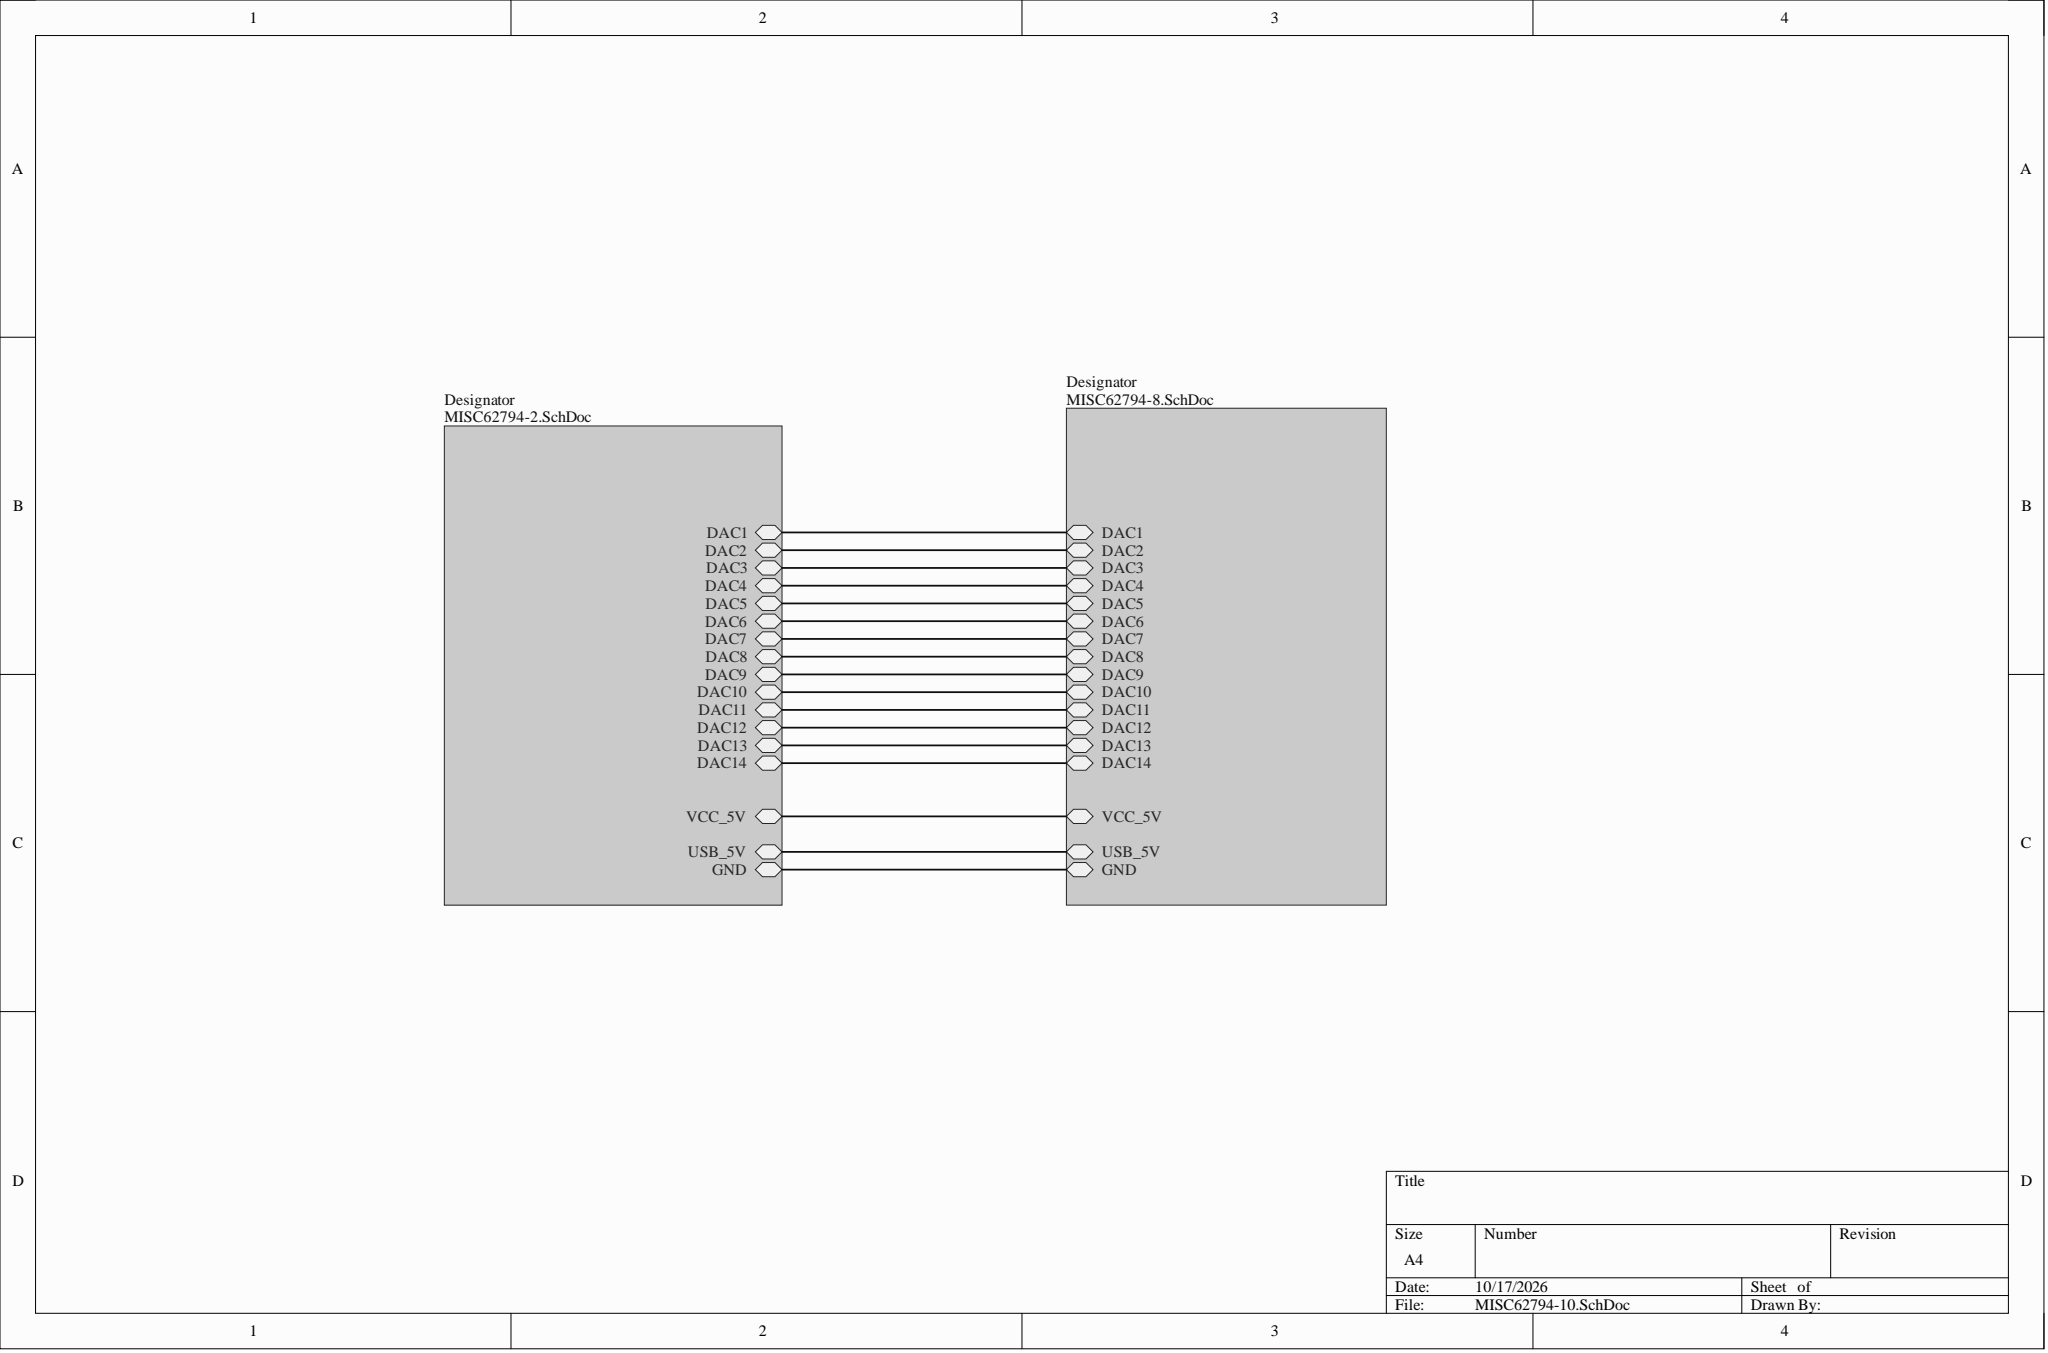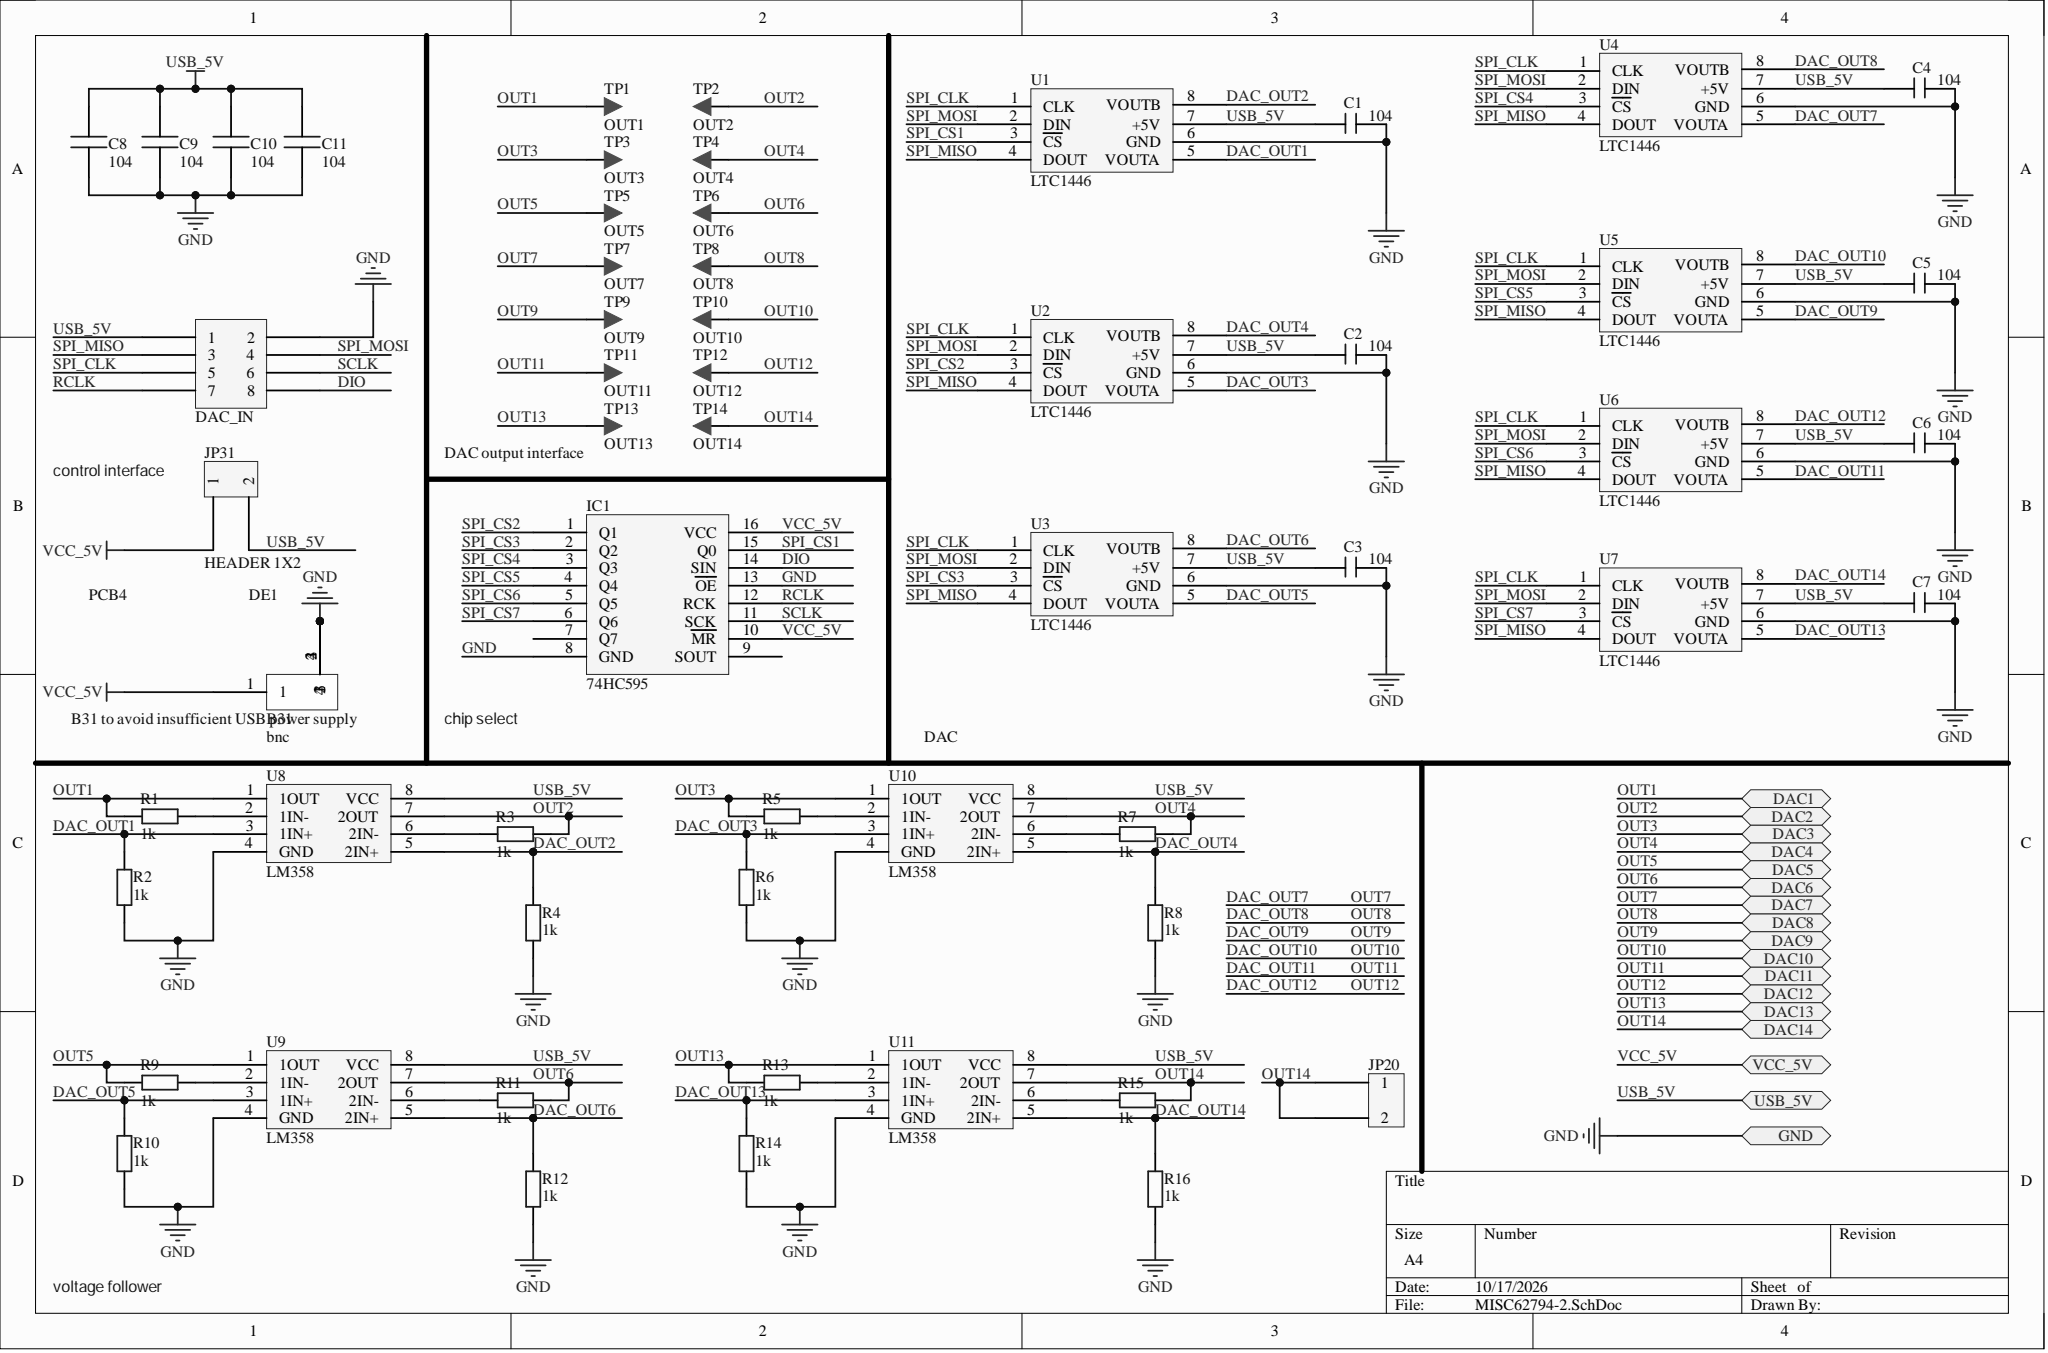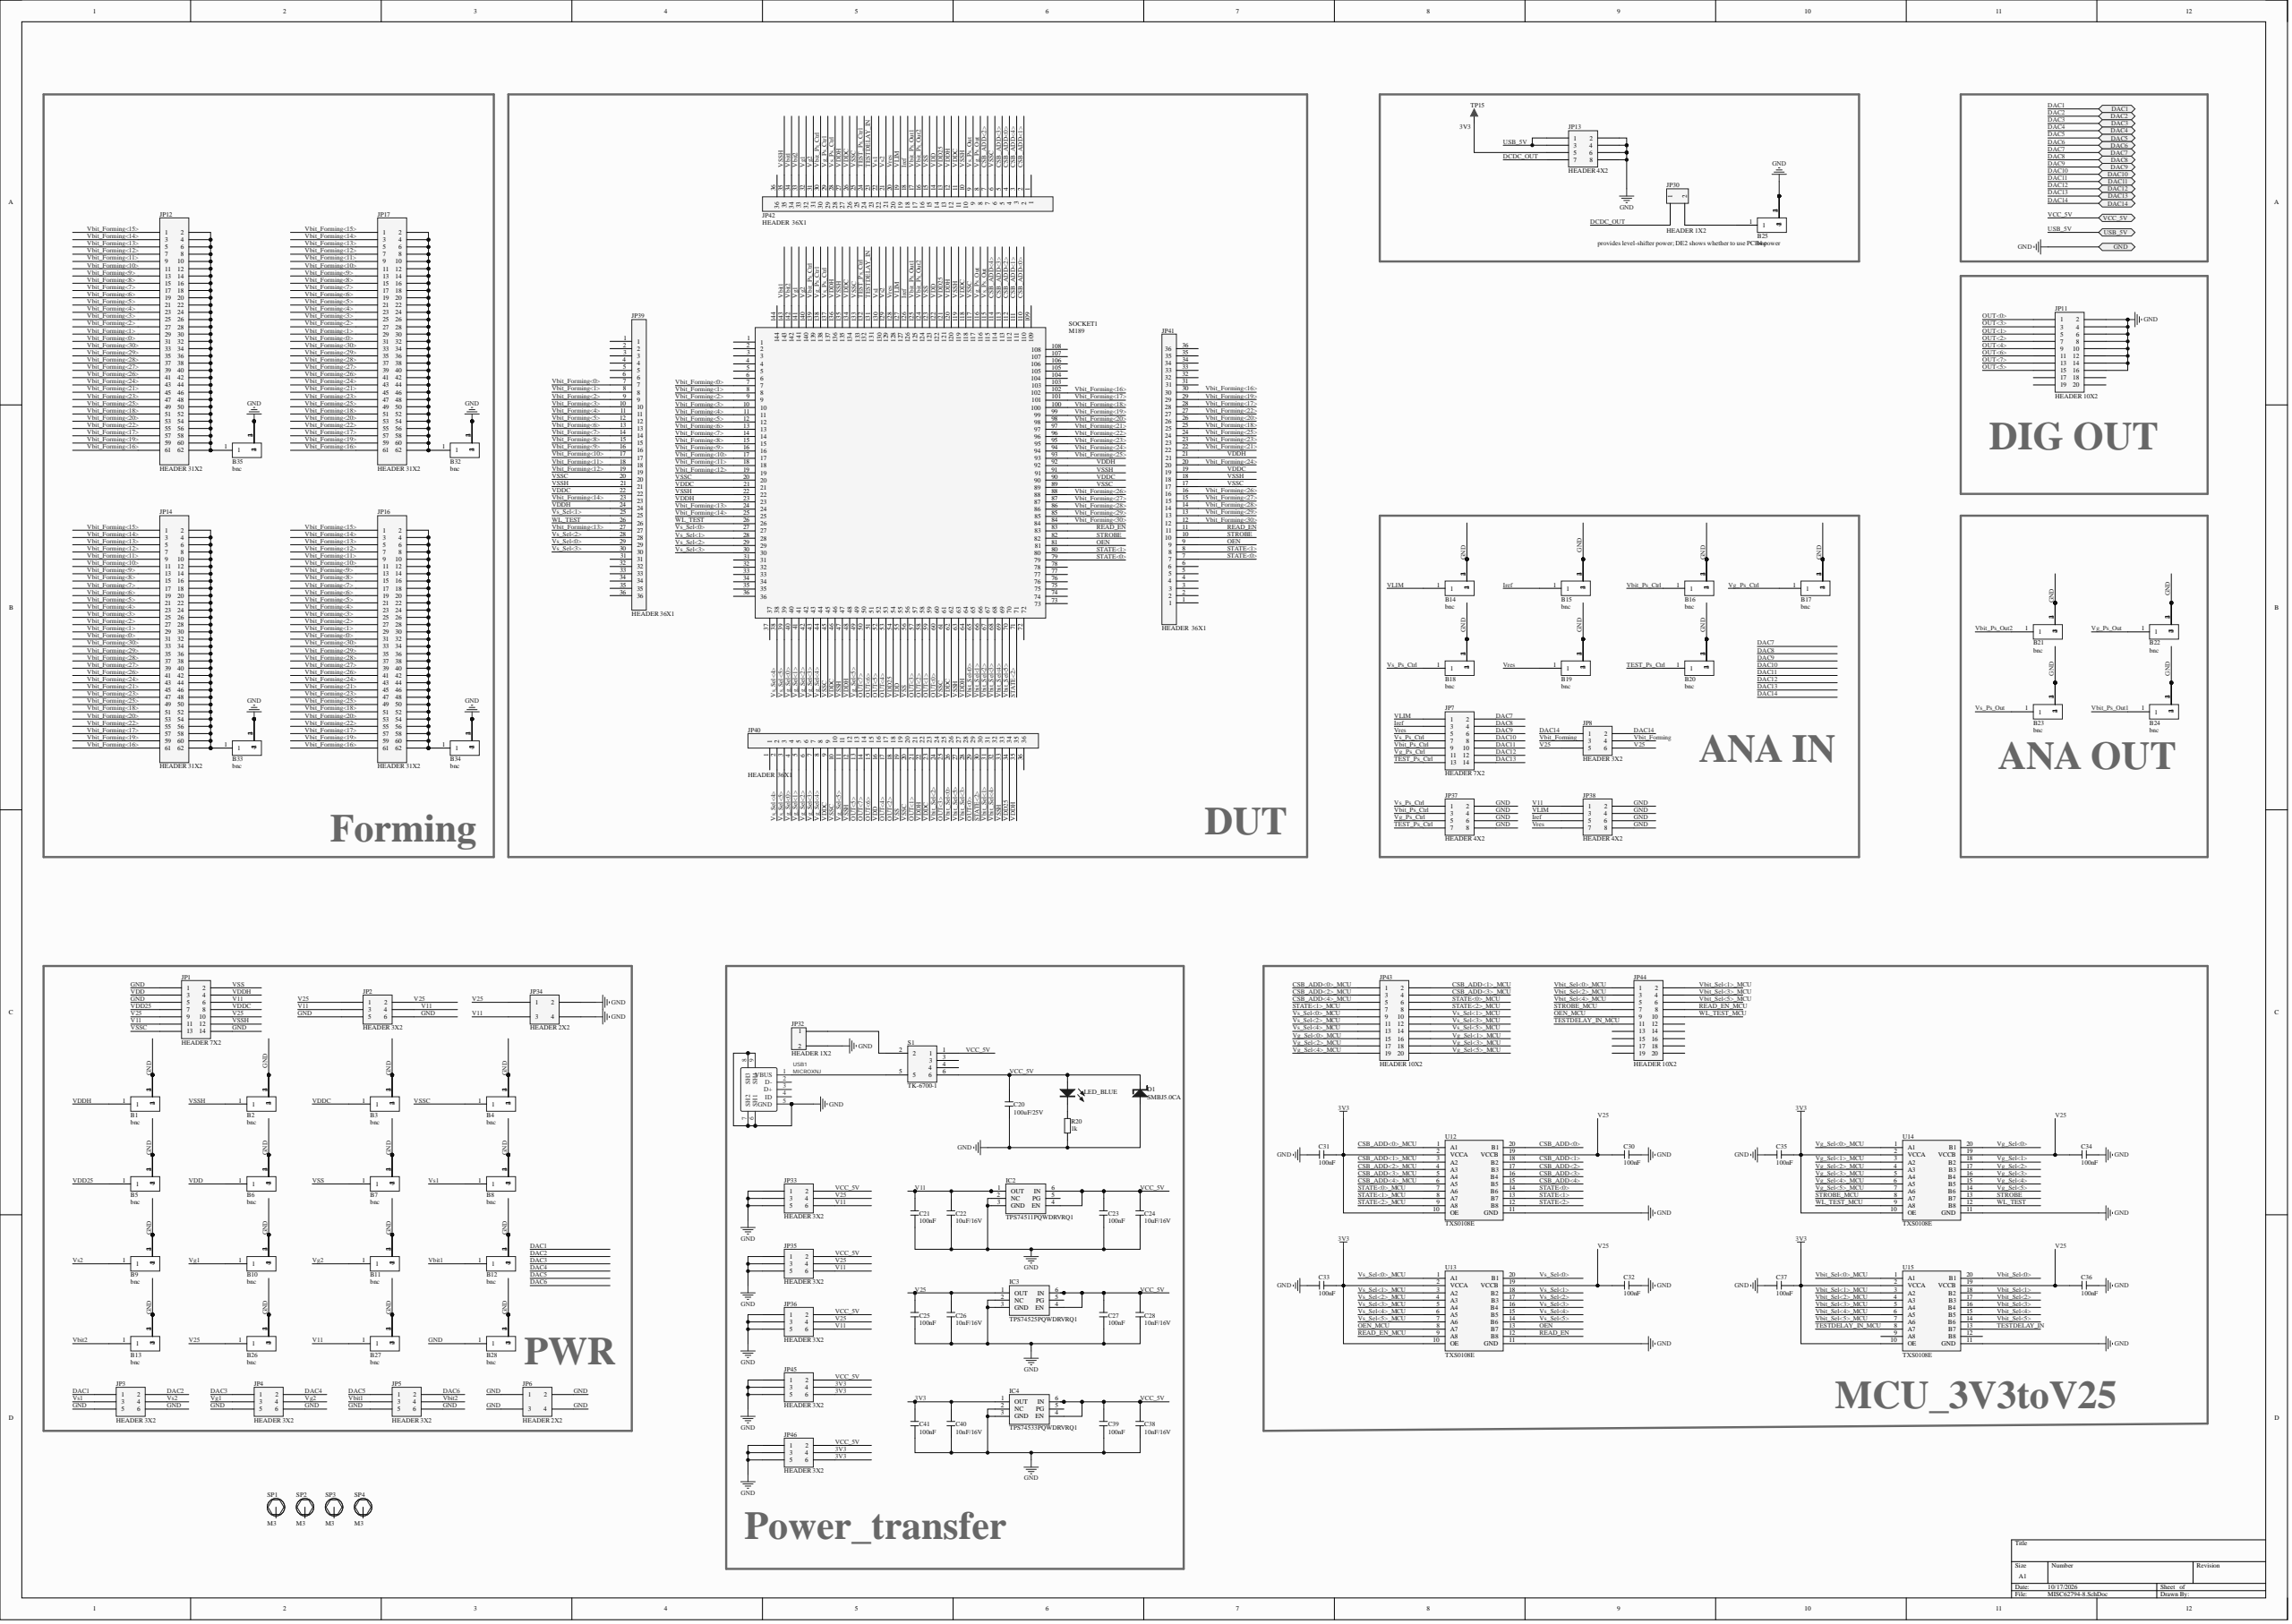Circuit board | Altium Designer | 158 parts | 185 nets
Bill of materials:
Comment,Description,Designator,Footprint,LibRef,Quantity
"bnc","bnc","B1, B2, B3, B4, B5, B6, B7, B8, B9, B10, B11, B12, B13, B14, B15, B16, B17, B18, B19, B20, B21, B22, B23, B24, B25, B26, B27, B28, B31, B32, B33, B34, B35","BNC-TH_DOSIN-801-0072","bnc","33"
"104","capacitor model","C1, C2, C3, C4, C5, C6, C7, C8, C9, C10, C11","0603C","CAP","11"
"100uF/25V","capacitor model","C20","EC-D6.3x7.7","CAP","1"
"100nF","capacitor model","C21, C23, C25, C27, C30, C31, C32, C33, C34, C35, C36, C37, C39, C41","0603C","CAP","14"
"10uF/16V","capacitor model","C22, C24","0603C","CAP","2"
"10nF/16V","capacitor model","C26, C28, C38, C40","0603C","CAP","4"
"SMBJ5.0CA","diode","D1","SMB","SMBJ5.0CA","1"
"DAC_IN","DAC_IN","DAC_IN","HDR2.54-LI-2x4P","DAC_IN","1"
"74HC595","IC","IC1","SOIC-16_L9.9-W3.9-P1.27-LS6.0-BL","74HC595","1"
"TPS74511PQWDRVRQ1","LDO","IC2","WSON-6_L2.0-W2.0-P0.65-BL-EP","TPS74511PQWDRVRQ1","1"
"TPS74525PQWDRVRQ1","LDO","IC3","WSON-6_L2.0-W2.0-P0.65-BL-EP","TPS74525PQWDRVRQ1","1"
"TPS74533PQWDRVRQ1","LDO","IC4","WSON-6_L2.0-W2.0-P0.65-BL-EP","TPS74533PQWDRVRQ1","1"
"HEADER 7X2","pin header","JP1, JP7","HDR2.54-LI-2x7P","HEADER 7X2","2"
"HEADER 3X2","pin header","JP2, JP3, JP4, JP5, JP8, JP33, JP35, JP36, JP45, JP46","HDR2.54-LI-2x3P","HEADER 3X2","10"
"HEADER 2X2","pin header","JP6","HDR2.54-LI-2x3P","HEADER 2X2","1"
"HEADER 10X2","pin header","JP11, JP43, JP44","HDR2.54-LI-2x10P","HEADER 10X2","3"
"HEADER 31X2","pin header","JP12, JP14, JP16, JP17","HDR2.54-LI-2x31P","HEADER 31X2","4"
"HEADER 4X2","pin header","JP13, JP37, JP38","HDR2.54-LI-2x4P","HEADER 4X2","3"
"HEADER 1X2","pin header","JP20, JP30, JP31, JP32","HDR2.54-LI-2P","HEADER 1X2","4"
"HEADER 2X2","pin header","JP34","HDR2.54-LI-2x2P","HEADER 2X2","1"
"HEADER 36X1","pin header","JP39","HDR2.54-LI-1x36P","HEADER 36X1","1"
"HEADER  36X1","pin header","JP40, JP41, JP42","HDR2.54-LI-1x36P","HEADER 36X1","3"
"LED","light-emitting diode","LED_BLUE","LED0805-R-RD","LED","1"
"1k","resistor model","R1, R2, R3, R4, R5, R6, R7, R8, R9, R10, R11, R12, R13, R14, R15, R16, R20","0603R","RES","17"
"TK-6700-1","six-pin self-locking switch","S1","SW-TH_6P-L8.0-W8.0-P2.50","switch6","1"
"M189","array","SOCKET1","YAMAICHI_IC51-1444-1354-7","M189_4K","1"
"M3","M3 interface","SP1, SP2, SP3, SP4","M3","M3","4"
"OUT1","TP","TP1","TP1.0","TP","1"
"OUT2","TP","TP2","TP1.0","TP","1"
"OUT3","TP","TP3","TP1.0","TP","1"
"OUT4","TP","TP4","TP1.0","TP","1"
"OUT5","TP","TP5","TP1.0","TP","1"
"OUT6","TP","TP6","TP1.0","TP","1"
"OUT7","TP","TP7","TP1.0","TP","1"
"OUT8","TP","TP8","TP1.0","TP","1"
"OUT9","TP","TP9","TP1.0","TP","1"
"OUT10","TP","TP10","TP1.0","TP","1"
"OUT11","TP","TP11","TP1.0","TP","1"
"OUT12","TP","TP12","TP1.0","TP","1"
"OUT13","TP","TP13","TP1.0","TP","1"
"OUT14","TP","TP14","TP1.0","TP","1"
"3V3","TP","TP15","TP1.0","TP","1"
"LTC1446","IC","U1, U2, U3, U4, U5, U6, U7","SO-8","LTC1446","7"
"LM358","IC","U8, U9, U10, U11","SO-8","LM358","4"
"TXS0108E","","U12, U13, U14, U15","TSSOP-20_L6.5-W4.4-P0.65-LS6.4-BL","TXS0108E","4"
"MICROXNJ","","USB1","MICRO-USB-SMD_MICROXNJ","MICROXNJ","1"
Netlist (Protel format):
[
B1
BNC-TH_DOSIN-801-0072
bnc



]
[
B2
BNC-TH_DOSIN-801-0072
bnc



]
[
B3
BNC-TH_DOSIN-801-0072
bnc



]
[
B4
BNC-TH_DOSIN-801-0072
bnc



]
[
B5
BNC-TH_DOSIN-801-0072
bnc



]
[
B6
BNC-TH_DOSIN-801-0072
bnc



]
[
B7
BNC-TH_DOSIN-801-0072
bnc



]
[
B8
BNC-TH_DOSIN-801-0072
bnc



]
[
B9
BNC-TH_DOSIN-801-0072
bnc



]
[
B10
BNC-TH_DOSIN-801-0072
bnc



]
[
B11
BNC-TH_DOSIN-801-0072
bnc



]
[
B12
BNC-TH_DOSIN-801-0072
bnc



]
[
B13
BNC-TH_DOSIN-801-0072
bnc



]
[
B14
BNC-TH_DOSIN-801-0072
bnc



]
[
B15
BNC-TH_DOSIN-801-0072
bnc



]
[
B16
BNC-TH_DOSIN-801-0072
bnc



]
[
B17
BNC-TH_DOSIN-801-0072
bnc



]
[
B18
BNC-TH_DOSIN-801-0072
bnc



]
[
B19
BNC-TH_DOSIN-801-0072
bnc



]
[
B20
BNC-TH_DOSIN-801-0072
bnc



]
[
B21
BNC-TH_DOSIN-801-0072
bnc



]
[
B22
BNC-TH_DOSIN-801-0072
bnc



]
[
B23
BNC-TH_DOSIN-801-0072
bnc



]
[
B24
BNC-TH_DOSIN-801-0072
bnc



]
[
B25
BNC-TH_DOSIN-801-0072
bnc



]
[
B26
BNC-TH_DOSIN-801-0072
bnc



]
[
B27
BNC-TH_DOSIN-801-0072
bnc



]
[
B28
BNC-TH_DOSIN-801-0072
bnc



]
[
B31
BNC-TH_DOSIN-801-0072
bnc



]
[
B32
BNC-TH_DOSIN-801-0072
bnc



]
[
B33
BNC-TH_DOSIN-801-0072
bnc



]
[
B34
BNC-TH_DOSIN-801-0072
bnc



]
[
B35
BNC-TH_DOSIN-801-0072
bnc



]
[
C1
0603C
104



]
[
C2
0603C
104



]
[
C3
0603C
104



]
[
C4
0603C
104



]
[
C5
0603C
104



]
[
C6
0603C
104



]
[
C7
0603C
104



]
[
C8
0603C
104



]
[
C9
0603C
104



]
[
C10
0603C
104



]
[
C11
0603C
104



]
[
C20
EC-D6.3x7.7
100uF/25V



]
[
C21
0603C
100nF



]
[
C22
0603C
10uF/16V



]
[
C23
0603C
100nF



]
[
C24
0603C
10uF/16V



]
[
C25
0603C
100nF



]
[
C26
0603C
10nF/16V



]
[
C27
0603C
100nF



]
[
C28
0603C
10nF/16V



]
[
C30
0603C
100nF



]
[
C31
0603C
100nF



]
[
C32
0603C
100nF



]
[
C33
0603C
100nF



]
[
C34
0603C
100nF



]
[
C35
0603C
100nF



]
[
C36
0603C
100nF



]
[
C37
0603C
100nF



]
[
C38
0603C
10nF/16V



]
[
C39
0603C
100nF



]
[
C40
0603C
10nF/16V



]
[
C41
0603C
100nF



]
[
D1
SMB
SMBJ5.0CA



]
[
DAC_IN
HDR2.54-LI-2x4P
DAC_IN



]
[
IC1
SOIC-16_L9.9-W3.9-P1.27-LS6.0-BL
74HC595



]
[
IC2
WSON-6_L2.0-W2.0-P0.65-BL-EP
TPS74511PQWDRVRQ1



]
[
IC3
WSON-6_L2.0-W2.0-P0.65-BL-EP
TPS74525PQWDRVRQ1



]
[
IC4
WSON-6_L2.0-W2.0-P0.65-BL-EP
TPS74533PQWDRVRQ1



]
[
JP1
HDR2.54-LI-2x7P
HEADER 7X2



]
[
JP2
HDR2.54-LI-2x3P
HEADER 3X2



]
[
JP3
HDR2.54-LI-2x3P
HEADER 3X2



]
[
JP4
HDR2.54-LI-2x3P
HEADER 3X2



]
[
JP5
HDR2.54-LI-2x3P
HEADER 3X2



]
[
JP6
HDR2.54-LI-2x3P
HEADER 2X2



]
[
JP7
HDR2.54-LI-2x7P
HEADER 7X2



]
[
JP8
HDR2.54-LI-2x3P
HEADER 3X2



]
[
JP11
HDR2.54-LI-2x10P
HEADER 10X2



]
[
JP12
HDR2.54-LI-2x31P
HEADER 31X2



]
[
JP13
HDR2.54-LI-2x4P
HEADER 4X2



]
[
JP14
HDR2.54-LI-2x31P
HEADER 31X2



]
[
JP16
HDR2.54-LI-2x31P
HEADER 31X2



]
[
JP17
HDR2.54-LI-2x31P
HEADER 31X2



]
[
JP20
HDR2.54-LI-2P
HEADER 1X2



]
[
JP30
HDR2.54-LI-2P
HEADER 1X2



]
[
JP31
HDR2.54-LI-2P
HEADER 1X2



]
[
JP32
HDR2.54-LI-2P
HEADER 1X2



]
[
JP33
HDR2.54-LI-2x3P
HEADER 3X2



]
[
JP34
HDR2.54-LI-2x2P
HEADER 2X2



]
[
JP35
HDR2.54-LI-2x3P
HEADER 3X2



]
[
JP36
HDR2.54-LI-2x3P
HEADER 3X2



]
[
JP37
HDR2.54-LI-2x4P
HEADER 4X2



]
[
JP38
HDR2.54-LI-2x4P
HEADER 4X2



]
[
JP39
HDR2.54-LI-1x36P
HEADER 36X1



]
[
JP40
HDR2.54-LI-1x36P
HEADER  36X1



]
[
JP41
HDR2.54-LI-1x36P
HEADER  36X1



]
[
JP42
HDR2.54-LI-1x36P
HEADER  36X1



]
[
JP43
HDR2.54-LI-2x10P
HEADER 10X2



]
[
JP44
HDR2.54-LI-2x10P
HEADER 10X2



]
[
JP45
HDR2.54-LI-2x3P
HEADER 3X2



]
[
JP46
HDR2.54-LI-2x3P
HEADER 3X2



]
[
LED_BLUE
LED0805-R-RD
LED



]
[
R1
0603R
1k



]
[
R2
0603R
1k



]
[
R3
0603R
1k



]
[
R4
0603R
1k



]
[
R5
0603R
1k



]
[
R6
0603R
1k



]
[
R7
0603R
1k



]
[
R8
0603R
1k



]
[
R9
0603R
1k



]
[
R10
0603R
1k



]
[
R11
0603R
1k



]
[
R12
0603R
1k



]
[
R13
0603R
1k



]
[
R14
0603R
1k



]
[
R15
0603R
1k



]
[
R16
0603R
1k



]
[
R20
0603R
1k



]
[
S1
SW-TH_6P-L8.0-W8.0-P2.50
TK-6700-1



]
[
SOCKET1
YAMAICHI_IC51-1444-1354-7
M189



]
[
SP1
M3
M3



]
[
SP2
M3
M3



]
[
SP3
M3
M3



]
[
SP4
M3
M3



]
[
TP1
TP1.0
OUT1



]
[
TP2
TP1.0
OUT2



]
[
TP3
TP1.0
OUT3



]
[
TP4
TP1.0
OUT4



]
[
TP5
TP1.0
OUT5



]
[
TP6
TP1.0
OUT6



]
[
TP7
TP1.0
OUT7



]
[
TP8
TP1.0
OUT8



]
[
TP9
TP1.0
OUT9



]
[
TP10
TP1.0
OUT10



]
[
TP11
TP1.0
OUT11



]
[
TP12
TP1.0
OUT12



]
[
TP13
TP1.0
OUT13



]
[
TP14
TP1.0
OUT14



]
[
TP15
TP1.0
3V3



]
[
U1
SO-8
LTC1446



]
[
U2
SO-8
LTC1446



]
[
U3
SO-8
LTC1446



]
[
U4
SO-8
LTC1446



]
[
U5
SO-8
LTC1446



]
[
U6
SO-8
LTC1446



]
[
U7
SO-8
LTC1446



]
[
U8
SO-8
LM358



]
[
U9
SO-8
LM358



]
[
U10
SO-8
LM358



]
[
U11
SO-8
LM358



]
[
U12
TSSOP-20_L6.5-W4.4-P0.65-LS6.4-BL
TXS0108E



]
[
U13
TSSOP-20_L6.5-W4.4-P0.65-LS6.4-BL
TXS0108E



]
[
U14
TSSOP-20_L6.5-W4.4-P0.65-LS6.4-BL
TXS0108E



]
[
U15
TSSOP-20_L6.5-W4.4-P0.65-LS6.4-BL
TXS0108E



]
[
USB1
MICRO-USB-SMD_MICROXNJ
MICROXNJ



]
(
WL_TEST_MCU
JP44-10
U14-9
)
(
WL_TEST
JP39-26
SOCKET1-26
U14-12
)
(
VSSH
B2-1
JP1-12
JP39-21
JP40-12
JP40-33
JP41-18
JP42-10
JP42-35
SOCKET1-22
SOCKET1-47
SOCKET1-63
SOCKET1-91
SOCKET1-119
SOCKET1-135
)
(
VSSC
B4-1
JP1-13
JP39-20
JP40-10
JP40-20
JP41-17
JP42-6
JP42-25
SOCKET1-20
SOCKET1-45
SOCKET1-61
SOCKET1-89
SOCKET1-117
SOCKET1-133
)
(
VSS
B7-1
JP1-2
JP40-19
JP42-15
SOCKET1-56
SOCKET1-123
)
(
Vs_Sel<5>_MCU
JP43-14
U13-7
)
(
Vs_Sel<5>
JP40-3
SOCKET1-39
U13-14
)
(
Vs_Sel<4>_MCU
JP43-13
U13-6
)
(
Vs_Sel<4>
JP40-2
SOCKET1-38
U13-15
)
(
Vs_Sel<3>_MCU
JP43-12
U13-5
)
(
Vs_Sel<3>
JP39-30
SOCKET1-30
U13-16
)
(
Vs_Sel<2>_MCU
JP43-11
U13-4
)
(
Vs_Sel<2>
JP39-28
SOCKET1-29
U13-17
)
(
Vs_Sel<1>_MCU
JP43-10
U13-3
)
(
Vs_Sel<1>
JP39-25
SOCKET1-28
U13-18
)
(
Vs_Sel<0>_MCU
JP43-9
U13-1
)
(
Vs_Sel<0>
JP39-29
SOCKET1-27
U13-20
)
(
Vs_Ps_Out
B23-1
JP42-9
SOCKET1-115
)
(
Vs_Ps_Ctrl
B18-1
JP7-7
JP37-1
JP42-28
SOCKET1-137
)
(
Vs2
B9-1
JP3-4
JP42-21
SOCKET1-129
)
(
Vs1
B8-1
JP3-3
JP42-22
SOCKET1-130
)
(
Vres
B19-1
JP7-5
JP38-7
JP42-20
SOCKET1-128
)
(
VLIM
B14-1
JP7-1
JP38-3
JP42-19
SOCKET1-127
)
(
Vg_Sel<5>_MCU
JP43-20
U14-7
)
(
Vg_Sel<5>
JP40-11
SOCKET1-49
U14-14
)
(
Vg_Sel<4>_MCU
JP43-19
U14-6
)
(
Vg_Sel<4>
JP40-8
SOCKET1-44
U14-15
)
(
Vg_Sel<3>_MCU
JP43-18
U14-5
)
(
Vg_Sel<3>
JP40-7
SOCKET1-43
U14-16
)
(
Vg_Sel<2>_MCU
JP43-17
U14-4
)
(
Vg_Sel<2>
JP40-6
SOCKET1-42
U14-17
)
(
Vg_Sel<1>_MCU
JP43-16
U14-3
)
(
Vg_Sel<1>
JP40-5
SOCKET1-41
U14-18
)
(
Vg_Sel<0>_MCU
JP43-15
U14-1
)
(
Vg_Sel<0>
JP40-4
SOCKET1-40
U14-20
)
(
Vg_Ps_Out
B22-1
JP42-8
SOCKET1-116
)
(
Vg_Ps_Ctrl
B17-1
JP7-11
JP37-5
JP42-29
SOCKET1-138
)
(
Vg2
B11-1
JP4-4
JP42-31
SOCKET1-140
)
(
Vg1
B10-1
JP4-3
JP42-32
SOCKET1-141
)
(
VDDH
B1-1
JP1-4
JP39-24
JP40-22
JP40-35
JP41-21
JP42-12
JP42-27
SOCKET1-23
SOCKET1-48
SOCKET1-64
SOCKET1-92
SOCKET1-120
SOCKET1-136
)
(
VDDC
B3-1
JP1-8
JP39-22
JP40-9
JP40-23
JP41-19
JP42-11
JP42-26
SOCKET1-21
SOCKET1-46
SOCKET1-62
SOCKET1-90
SOCKET1-118
SOCKET1-134
)
(
VDD25
B5-1
JP1-7
JP40-34
JP42-13
SOCKET1-54
SOCKET1-121
)
(
VDD
B6-1
JP1-3
JP40-16
JP42-14
SOCKET1-55
SOCKET1-122
)
(
VCC_5V
B31-1
C20-1
C23-1
C24-1
C27-1
C28-1
C38-1
C39-1
D1-1
IC1-10
IC1-16
IC2-4
IC2-6
IC3-4
IC3-6
IC4-4
IC4-6
JP31-1
JP33-2
JP35-2
JP36-2
JP45-2
JP46-2
LED_BLUE-1
S1-1
S1-6
)
(
Vbit_Sel<5>_MCU
JP44-6
U15-7
)
(
Vbit_Sel<5>
JP40-27
SOCKET1-70
U15-14
)
(
Vbit_Sel<4>_MCU
JP44-5
U15-6
)
(
Vbit_Sel<4>
JP40-32
SOCKET1-69
U15-15
)
(
Vbit_Sel<3>_MCU
JP44-4
U15-5
)
(
Vbit_Sel<3>
JP40-28
SOCKET1-68
U15-16
)
(
Vbit_Sel<2>_MCU
JP44-3
U15-4
)
(
Vbit_Sel<2>
JP40-24
SOCKET1-67
U15-17
)
(
Vbit_Sel<1>_MCU
JP44-2
U15-3
)
(
Vbit_Sel<1>
JP40-31
SOCKET1-66
U15-18
)
(
Vbit_Sel<0>_MCU
JP44-1
U15-1
)
(
Vbit_Sel<0>
JP40-26
SOCKET1-65
U15-20
)
(
Vbit_Ps_Out2
B21-1
JP42-16
SOCKET1-124
)
(
Vbit_Ps_Out1
B24-1
JP42-17
SOCKET1-125
)
(
Vbit_Ps_Ctrl
B16-1
JP7-9
JP37-3
JP42-30
SOCKET1-139
)
(
Vbit_Forming<30>
JP12-33
JP14-33
JP16-33
JP17-33
JP41-12
SOCKET1-84
)
(
Vbit_Forming<29>
JP12-35
JP14-35
JP16-35
JP17-35
JP41-13
SOCKET1-85
)
(
Vbit_Forming<28>
JP12-37
JP14-37
JP16-37
JP17-37
JP41-14
SOCKET1-86
)
(
Vbit_Forming<27>
JP12-39
JP14-39
JP16-39
JP17-39
JP41-15
SOCKET1-87
)
(
Vbit_Forming<26>
JP12-41
JP14-41
JP16-41
JP17-41
JP41-16
SOCKET1-88
)
(
Vbit_Forming<25>
JP12-49
JP14-49
JP16-49
JP17-49
JP41-24
SOCKET1-93
)
(
Vbit_Forming<24>
JP12-43
JP14-43
JP16-43
JP17-43
JP41-20
SOCKET1-94
)
(
Vbit_Forming<23>
JP12-47
JP14-47
JP16-47
JP17-47
JP41-23
SOCKET1-95
)
(
Vbit_Forming<22>
JP12-55
JP14-55
JP16-55
JP17-55
JP41-27
SOCKET1-96
)
(
Vbit_Forming<21>
JP12-45
JP14-45
JP16-45
JP17-45
JP41-22
SOCKET1-97
)
(
Vbit_Forming<20>
JP12-53
JP14-53
JP16-53
JP17-53
JP41-26
SOCKET1-98
)
(
Vbit_Forming<19>
JP12-59
JP14-59
JP16-59
JP17-59
JP41-29
SOCKET1-99
)
(
Vbit_Forming<18>
JP12-51
JP14-51
JP16-51
JP17-51
JP41-25
SOCKET1-100
)
(
Vbit_Forming<17>
JP12-57
JP14-57
JP16-57
JP17-57
JP41-28
SOCKET1-101
)
(
Vbit_Forming<16>
JP12-61
JP14-61
JP16-61
JP17-61
JP41-30
SOCKET1-102
)
(
Vbit_Forming<15>
JP12-1
JP14-1
JP16-1
JP17-1
)
(
Vbit_Forming<14>
JP12-3
JP14-3
JP16-3
JP17-3
JP39-23
SOCKET1-25
)
(
Vbit_Forming<13>
JP12-5
JP14-5
JP16-5
JP17-5
JP39-27
SOCKET1-24
)
(
Vbit_Forming<12>
JP12-7
JP14-7
JP16-7
JP17-7
JP39-19
SOCKET1-19
)
(
Vbit_Forming<11>
JP12-9
JP14-9
JP16-9
JP17-9
JP39-18
SOCKET1-18
)
(
Vbit_Forming<10>
JP12-11
JP14-11
JP16-11
JP17-11
JP39-17
SOCKET1-17
)
(
Vbit_Forming<9>
JP12-13
JP14-13
JP16-13
JP17-13
JP39-16
SOCKET1-16
)
(
Vbit_Forming<8>
JP12-15
JP14-15
JP16-15
JP17-15
JP39-15
SOCKET1-15
)
(
Vbit_Forming<7>
JP12-17
JP14-17
JP16-17
JP17-17
JP39-14
SOCKET1-14
)
(
Vbit_Forming<6>
JP12-19
JP14-19
JP16-19
JP17-19
JP39-13
SOCKET1-13
)
(
Vbit_Forming<5>
JP12-21
JP14-21
JP16-21
JP17-21
JP39-12
SOCKET1-12
)
(
Vbit_Forming<4>
JP12-23
JP14-23
JP16-23
JP17-23
JP39-11
SOCKET1-11
)
(
Vbit_Forming<3>
JP12-25
JP14-25
JP16-25
JP17-25
JP39-10
SOCKET1-10
)
(
Vbit_Forming<2>
JP12-27
JP14-27
JP16-27
JP17-27
JP39-9
SOCKET1-9
)
(
Vbit_Forming<1>
JP12-29
JP14-29
JP16-29
JP17-29
JP39-8
SOCKET1-8
)
(
Vbit_Forming<0>
JP12-31
JP14-31
JP16-31
JP17-31
JP39-7
SOCKET1-7
)
(
Vbit_Forming
JP8-3
JP8-4
)
(
Vbit2
B13-1
JP5-4
JP42-33
SOCKET1-142
)
(
Vbit1
B12-1
JP5-3
JP42-34
SOCKET1-143
)
(
V25
B26-1
C25-1
C26-1
C30-2
C32-2
C34-2
C36-2
IC3-1
JP1-9
JP1-10
JP2-1
JP2-2
JP8-5
JP8-6
JP33-4
JP34-1
JP35-4
JP36-4
U12-19
U13-19
U14-19
U15-19
)
(
V11
B27-1
C21-1
C22-1
IC2-1
JP1-6
JP1-11
JP2-3
JP2-4
JP33-6
JP34-3
JP35-6
JP36-6
JP38-1
)
(
USB_5V
C1-2
C2-2
C3-2
C4-2
C5-2
C6-2
C7-2
C8-1
C9-1
C10-1
C11-1
DAC_IN-1
JP13-1
JP13-3
JP31-2
U1-7
U2-7
U3-7
U4-7
U5-7
U6-7
U7-7
U8-8
U9-8
U10-8
U11-8
)
(
TESTDELAY_IN_MCU
JP44-11
U15-8
)
(
TESTDELAY_IN
JP42-23
SOCKET1-131
U15-13
)
(
TEST_Ps_Ctrl
B20-1
JP7-13
JP37-7
JP42-24
SOCKET1-132
)
(
STROBE_MCU
JP44-7
U14-8
)
(
STROBE
JP41-10
SOCKET1-82
U14-13
)
(
STATE<2>_MCU
JP43-8
U12-9
)
(
STATE<2>
JP40-30
SOCKET1-71
U12-12
)
(
STATE<1>_MCU
JP43-7
U12-8
)
(
STATE<1>
JP41-8
SOCKET1-80
U12-13
)
(
STATE<0>_MCU
JP43-6
U12-7
)
(
STATE<0>
JP41-7
SOCKET1-79
U12-14
)
(
SPI_MOSI
DAC_IN-4
U1-2
U2-2
U3-2
U4-2
U5-2
U6-2
U7-2
)
(
SPI_MISO
DAC_IN-3
U1-4
U2-4
U3-4
U4-4
U5-4
U6-4
U7-4
)
(
SPI_CS7
IC1-6
U7-3
)
(
SPI_CS6
IC1-5
U6-3
)
(
SPI_CS5
IC1-4
U5-3
)
(
SPI_CS4
IC1-3
U4-3
)
(
SPI_CS3
IC1-2
U3-3
)
(
SPI_CS2
IC1-1
U2-3
)
(
SPI_CS1
IC1-15
U1-3
)
(
SPI_CLK
DAC_IN-5
U1-1
U2-1
U3-1
U4-1
U5-1
U6-1
U7-1
)
(
SCLK
DAC_IN-6
IC1-11
)
(
READ_EN_MCU
JP44-8
U13-9
)
(
READ_EN
JP41-11
SOCKET1-83
U13-12
)
(
RCLK
DAC_IN-7
IC1-12
)
(
OUT<7>
JP11-13
JP40-14
SOCKET1-50
)
(
OUT<6>
JP11-11
JP40-15
SOCKET1-51
)
(
OUT<5>
JP11-15
JP40-13
SOCKET1-52
)
(
OUT<4>
JP11-9
JP40-17
SOCKET1-53
)
(
OUT<3>
JP11-3
JP40-25
SOCKET1-57
)
(
OUT<2>
JP11-7
JP40-18
SOCKET1-58
)
(
OUT<1>
JP11-5
JP40-21
SOCKET1-59
)
(
OUT<0>
JP11-1
JP40-29
SOCKET1-60
)
(
OEN_MCU
JP44-9
U13-8
)
(
OEN
JP41-9
SOCKET1-81
U13-13
)
(
NetS1_5
S1-5
USB1-1
)
(
NetR15_2
R15-2
U11-6
)
(
NetR13_1
R13-1
U11-2
)
(
NetR11_2
R11-2
U9-6
)
(
NetR9_1
R9-1
U9-2
)
(
NetR7_2
R7-2
U10-6
)
(
NetR5_1
R5-1
U10-2
)
(
NetR3_2
R3-2
U8-6
)
(
NetR1_1
R1-1
U8-2
)
(
NetLED_BLUE_2
LED_BLUE-2
R20-1
)
(
NetJP32_1
JP32-1
S1-2
)
(
NetJP13_5
JP13-5
TP15-1
)
(
NetB35_1
B35-1
JP12-2
JP12-4
JP12-6
JP12-8
JP12-10
JP12-12
JP12-14
JP12-16
JP12-18
JP12-20
JP12-22
JP12-24
JP12-26
JP12-28
JP12-30
JP12-32
JP12-34
JP12-36
JP12-38
JP12-40
JP12-42
JP12-44
JP12-46
JP12-48
JP12-50
JP12-52
JP12-54
JP12-56
JP12-58
JP12-60
JP12-62
)
(
NetB34_1
B34-1
JP16-2
JP16-4
JP16-6
JP16-8
JP16-10
JP16-12
JP16-14
JP16-16
JP16-18
JP16-20
JP16-22
JP16-24
JP16-26
JP16-28
JP16-30
JP16-32
JP16-34
JP16-36
JP16-38
JP16-40
JP16-42
JP16-44
JP16-46
JP16-48
JP16-50
JP16-52
JP16-54
JP16-56
JP16-58
JP16-60
JP16-62
)
(
NetB33_1
B33-1
JP14-2
JP14-4
JP14-6
JP14-8
JP14-10
JP14-12
JP14-14
JP14-16
JP14-18
JP14-20
JP14-22
JP14-24
JP14-26
JP14-28
JP14-30
JP14-32
JP14-34
JP14-36
JP14-38
JP14-40
JP14-42
JP14-44
JP14-46
JP14-48
JP14-50
JP14-52
JP14-54
JP14-56
JP14-58
JP14-60
JP14-62
)
(
NetB32_1
B32-1
JP17-2
JP17-4
JP17-6
JP17-8
JP17-10
JP17-12
JP17-14
JP17-16
JP17-18
JP17-20
JP17-22
JP17-24
JP17-26
JP17-28
JP17-30
JP17-32
JP17-34
JP17-36
JP17-38
JP17-40
JP17-42
JP17-44
JP17-46
JP17-48
JP17-50
JP17-52
JP17-54
JP17-56
JP17-58
JP17-60
JP17-62
)
(
NetB25_1
B25-1
JP30-2
)
(
Iref
B15-1
JP7-3
JP38-5
JP42-18
SOCKET1-126
)
(
GND
B1-2
B1-3
B1-4
B2-2
B2-3
B2-4
B3-2
B3-3
B3-4
B4-2
B4-3
B4-4
B5-2
B5-3
B5-4
B6-2
B6-3
B6-4
B7-2
B7-3
B7-4
B8-2
B8-3
B8-4
B9-2
B9-3
B9-4
B10-2
B10-3
B10-4
B11-2
B11-3
B11-4
B12-2
B12-3
B12-4
B13-2
B13-3
B13-4
B14-2
B14-3
B14-4
B15-2
B15-3
B15-4
B16-2
B16-3
B16-4
B17-2
B17-3
B17-4
B18-2
B18-3
B18-4
B19-2
B19-3
B19-4
B20-2
B20-3
B20-4
B21-2
B21-3
B21-4
B22-2
B22-3
B22-4
B23-2
B23-3
B23-4
B24-2
B24-3
B24-4
B25-2
B25-3
B25-4
B26-2
B26-3
B26-4
B27-2
B27-3
B27-4
B28-1
B28-2
B28-3
B28-4
B31-2
B31-3
B31-4
B32-2
B32-3
B32-4
B33-2
B33-3
B33-4
B34-2
B34-3
B34-4
B35-2
B35-3
B35-4
C1-1
C2-1
C3-1
C4-1
C5-1
C6-1
C7-1
C8-2
C9-2
C10-2
C11-2
C20-2
C21-2
C22-2
C23-2
C24-2
C25-2
C26-2
C27-2
C28-2
C30-1
C31-2
C32-1
C33-2
C34-1
C35-2
C36-1
C37-2
C38-2
C39-2
C40-2
C41-2
D1-2
DAC_IN-2
IC1-8
IC1-13
IC2-2
IC2-3
IC3-2
IC3-3
IC4-2
IC4-3
JP1-1
JP1-5
JP1-14
JP2-5
JP2-6
JP3-5
JP3-6
JP4-5
JP4-6
JP5-5
JP5-6
JP6-1
JP6-2
JP6-3
JP6-4
JP11-2
JP11-4
JP11-6
JP11-8
JP11-10
JP11-12
JP11-14
JP11-16
JP13-2
JP13-4
JP13-6
JP13-8
JP32-2
JP33-1
JP33-3
JP33-5
JP34-2
JP34-4
JP35-1
JP35-3
JP35-5
JP36-1
JP36-3
JP36-5
JP37-2
JP37-4
JP37-6
JP37-8
JP38-2
JP38-4
JP38-6
JP38-8
JP45-1
JP45-3
JP45-5
JP46-1
JP46-3
JP46-5
R2-2
R4-2
R6-2
R8-2
R10-2
R12-2
R14-2
R16-2
R20-2
U1-6
U2-6
U3-6
U4-6
U5-6
U6-6
U7-6
U8-4
U9-4
U10-4
U11-4
U12-11
U13-11
U14-11
U15-11
USB1-5
USB1-6
USB1-7
USB1-8
USB1-9
)
(
DIO
DAC_IN-8
IC1-14
)
(
DCDC_OUT
JP13-7
JP30-1
)
(
DAC_OUT14
R16-1
U7-8
U11-5
)
(
DAC_OUT13
R14-1
U7-5
U11-3
)
(
DAC_OUT6
R12-1
U3-8
U9-5
)
(
DAC_OUT5
R10-1
U3-5
U9-3
)
(
DAC_OUT4
R8-1
U2-8
U10-5
)
(
DAC_OUT3
R6-1
U2-5
U10-3
)
(
DAC_OUT2
R4-1
U1-8
U8-5
)
(
DAC_OUT1
R2-1
U1-5
U8-3
)
(
DAC14
JP8-1
JP8-2
JP20-1
JP20-2
R15-1
TP14-1
U11-7
)
(
DAC13
JP7-14
R13-2
TP13-1
U11-1
)
(
DAC12
JP7-12
TP12-1
U6-8
)
(
DAC11
JP7-10
TP11-1
U6-5
)
(
DAC10
JP7-8
TP10-1
U5-8
)
(
DAC9
JP7-6
TP9-1
U5-5
)
(
DAC8
JP7-4
TP8-1
U4-8
)
(
DAC7
JP7-2
TP7-1
U4-5
)
(
DAC6
JP5-2
R11-1
TP6-1
U9-7
)
(
DAC5
JP5-1
R9-2
TP5-1
U9-1
)
(
DAC4
JP4-2
R7-1
TP4-1
U10-7
)
(
DAC3
JP4-1
R5-2
TP3-1
U10-1
)
(
DAC2
JP3-2
R3-1
TP2-1
U8-7
)
(
DAC1
JP3-1
R1-2
TP1-1
U8-1
)
(
CSB_ADD<4>_MCU
JP43-5
U12-6
)
(
CSB_ADD<4>
JP42-3
SOCKET1-114
U12-15
)
(
CSB_ADD<3>_MCU
JP43-4
U12-5
)
(
CSB_ADD<3>
JP42-5
SOCKET1-113
U12-16
)
(
CSB_ADD<2>_MCU
JP43-3
U12-4
)
(
CSB_ADD<2>
JP42-7
SOCKET1-112
U12-17
)
(
CSB_ADD<1>_MCU
JP43-2
U12-3
)
(
CSB_ADD<1>
JP42-2
SOCKET1-111
U12-18
)
(
CSB_ADD<0>_MCU
JP43-1
U12-1
)
(
CSB_ADD<0>
JP42-4
SOCKET1-110
U12-20
)
(
3V3
C31-1
C33-1
C35-1
C37-1
C40-1
C41-1
IC4-1
JP45-4
JP45-6
JP46-4
JP46-6
U12-2
U12-10
U13-2
U13-10
U14-2
U14-10
U15-2
U15-10
)